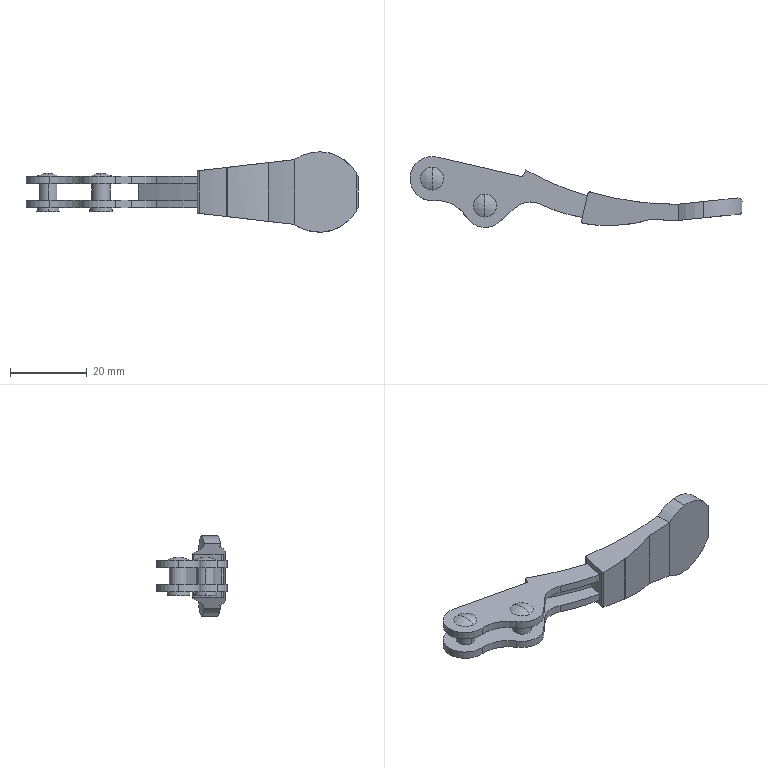Part | STEP file | 11-HANDLE_MC01-S311 | 1 solid | 60 faces | box 86.6 x 18.497 x 20.98 mm | volume 5479 mm3 | cylinder 34 | plane 22 | sphere 4 | commonest cylinder face diameters 1 x4 4.85 x4 5.85 x4 11.5 x4 22.26 x3 11.4 x2